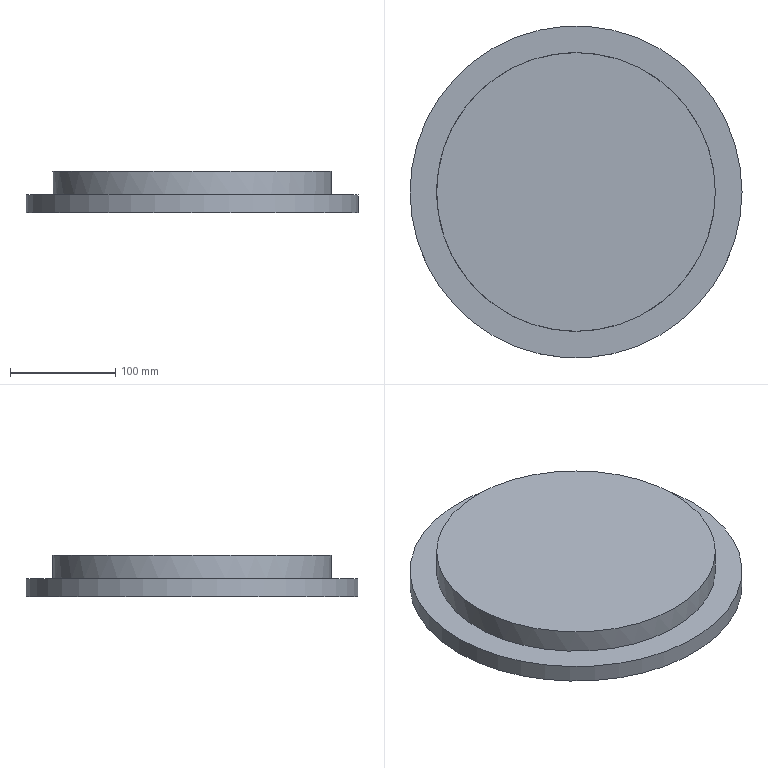Part | NX | features CYLINDER 3, DATUM_CSYS 1, Delete Body 1, LINKED_BODY 1, SCALE 1, UNITE 1 | 1 solid | 7 faces | box 315 x 315 x 39.375 mm | volume 2172802 mm3 | plane 4 | cylinder 3 | commonest cylinder face diameters 168.75 x1 264.375 x1 315 x1
STEP:
#1=CARTESIAN_POINT('',(-234.395,-2029.479,187.25));
#2=VERTEX_POINT('',#1);
#3=CARTESIAN_POINT('',(-366.582,-2029.479,187.25));
#4=DIRECTION('',(0.,0.,1.));
#5=DIRECTION('',(1.,0.,0.));
#6=AXIS2_PLACEMENT_3D('',#3,#4,#5);
#7=CIRCLE('',#6,132.188);
#8=EDGE_CURVE('',#2,#2,#7,.T.);
#9=ORIENTED_EDGE('',*,*,#8,.F.);
#10=EDGE_LOOP('',(#9));
#11=FACE_BOUND('',#10,.T.);
#12=CARTESIAN_POINT('',(-524.082,-2029.479,187.25));
#13=VERTEX_POINT('',#12);
#14=CARTESIAN_POINT('',(-366.582,-2029.479,187.25));
#15=DIRECTION('',(0.,0.,-1.));
#16=DIRECTION('',(-1.,0.,0.));
#17=AXIS2_PLACEMENT_3D('',#14,#15,#16);
#18=CIRCLE('',#17,157.5);
#19=EDGE_CURVE('',#13,#13,#18,.T.);
#20=ORIENTED_EDGE('',*,*,#19,.F.);
#21=EDGE_LOOP('',(#20));
#22=FACE_BOUND('',#21,.T.);
#23=CARTESIAN_POINT('',(-366.582,-2029.479,187.25));
#24=DIRECTION('',(0.,0.,1.));
#25=DIRECTION('',(1.,0.,0.));
#26=AXIS2_PLACEMENT_3D('',#23,#24,#25);
#27=PLANE('',#26);
#28=ADVANCED_FACE('',(#11,#22),#27,.T.);
#29=CARTESIAN_POINT('',(-282.207,-2029.479,170.375));
#30=VERTEX_POINT('',#29);
#31=CARTESIAN_POINT('',(-366.582,-2029.479,170.375));
#32=DIRECTION('',(0.,0.,1.));
#33=DIRECTION('',(1.,0.,0.));
#34=AXIS2_PLACEMENT_3D('',#31,#32,#33);
#35=CIRCLE('',#34,84.375);
#36=EDGE_CURVE('',#30,#30,#35,.T.);
#37=ORIENTED_EDGE('',*,*,#36,.T.);
#38=EDGE_LOOP('',(#37));
#39=FACE_BOUND('',#38,.T.);
#40=CARTESIAN_POINT('',(-209.082,-2029.479,170.375));
#41=VERTEX_POINT('',#40);
#42=CARTESIAN_POINT('',(-366.582,-2029.479,170.375));
#43=DIRECTION('',(0.,0.,1.));
#44=DIRECTION('',(1.,0.,0.));
#45=AXIS2_PLACEMENT_3D('',#42,#43,#44);
#46=CIRCLE('',#45,157.5);
#47=EDGE_CURVE('',#41,#41,#46,.T.);
#48=ORIENTED_EDGE('',*,*,#47,.F.);
#49=EDGE_LOOP('',(#48));
#50=FACE_BOUND('',#49,.T.);
#51=CARTESIAN_POINT('',(-366.582,-2029.479,170.375));
#52=DIRECTION('',(0.,0.,-1.));
#53=DIRECTION('',(-1.,0.,0.));
#54=AXIS2_PLACEMENT_3D('',#51,#52,#53);
#55=PLANE('',#54);
#56=ADVANCED_FACE('',(#39,#50),#55,.T.);
#57=ORIENTED_EDGE('',*,*,#19,.T.);
#58=EDGE_LOOP('',(#57));
#59=FACE_BOUND('',#58,.T.);
#60=ORIENTED_EDGE('',*,*,#47,.T.);
#61=EDGE_LOOP('',(#60));
#62=FACE_BOUND('',#61,.T.);
#63=CARTESIAN_POINT('',(-366.582,-2029.479,170.375));
#64=DIRECTION('',(0.,0.,1.));
#65=DIRECTION('',(1.,0.,0.));
#66=AXIS2_PLACEMENT_3D('',#63,#64,#65);
#67=CYLINDRICAL_SURFACE('',#66,157.5);
#68=ADVANCED_FACE('',(#59,#62),#67,.T.);
#69=CARTESIAN_POINT('',(-498.77,-2029.479,209.75));
#70=VERTEX_POINT('',#69);
#71=CARTESIAN_POINT('',(-366.582,-2029.479,209.75));
#72=DIRECTION('',(0.,0.,-1.));
#73=DIRECTION('',(-1.,0.,0.));
#74=AXIS2_PLACEMENT_3D('',#71,#72,#73);
#75=CIRCLE('',#74,132.188);
#76=EDGE_CURVE('',#70,#70,#75,.T.);
#77=ORIENTED_EDGE('',*,*,#76,.F.);
#78=EDGE_LOOP('',(#77));
#79=FACE_BOUND('',#78,.T.);
#80=CARTESIAN_POINT('',(-366.582,-2029.479,209.75));
#81=DIRECTION('',(0.,0.,1.));
#82=DIRECTION('',(1.,0.,0.));
#83=AXIS2_PLACEMENT_3D('',#80,#81,#82);
#84=PLANE('',#83);
#85=ADVANCED_FACE('',(#79),#84,.T.);
#86=ORIENTED_EDGE('',*,*,#8,.T.);
#87=EDGE_LOOP('',(#86));
#88=FACE_BOUND('',#87,.T.);
#89=ORIENTED_EDGE('',*,*,#76,.T.);
#90=EDGE_LOOP('',(#89));
#91=FACE_BOUND('',#90,.T.);
#92=CARTESIAN_POINT('',(-366.582,-2029.479,170.375));
#93=DIRECTION('',(0.,0.,1.));
#94=DIRECTION('',(1.,0.,0.));
#95=AXIS2_PLACEMENT_3D('',#92,#93,#94);
#96=CYLINDRICAL_SURFACE('',#95,132.188);
#97=ADVANCED_FACE('',(#88,#91),#96,.T.);
#98=CARTESIAN_POINT('',(-450.957,-2029.479,187.25));
#99=VERTEX_POINT('',#98);
#100=CARTESIAN_POINT('',(-366.582,-2029.479,187.25));
#101=DIRECTION('',(0.,0.,-1.));
#102=DIRECTION('',(-1.,0.,0.));
#103=AXIS2_PLACEMENT_3D('',#100,#101,#102);
#104=CIRCLE('',#103,84.375);
#105=EDGE_CURVE('',#99,#99,#104,.F.);
#106=ORIENTED_EDGE('',*,*,#105,.F.);
#107=EDGE_LOOP('',(#106));
#108=FACE_BOUND('',#107,.T.);
#109=CARTESIAN_POINT('',(-366.582,-2029.479,187.25));
#110=DIRECTION('',(0.,0.,1.));
#111=DIRECTION('',(1.,0.,0.));
#112=AXIS2_PLACEMENT_3D('',#109,#110,#111);
#113=PLANE('',#112);
#114=ADVANCED_FACE('',(#108),#113,.F.);
#115=ORIENTED_EDGE('',*,*,#105,.T.);
#116=EDGE_LOOP('',(#115));
#117=FACE_BOUND('',#116,.T.);
#118=ORIENTED_EDGE('',*,*,#36,.F.);
#119=EDGE_LOOP('',(#118));
#120=FACE_BOUND('',#119,.T.);
#121=CARTESIAN_POINT('',(-366.582,-2029.479,170.375));
#122=DIRECTION('',(0.,0.,1.));
#123=DIRECTION('',(1.,0.,0.));
#124=AXIS2_PLACEMENT_3D('',#121,#122,#123);
#125=CYLINDRICAL_SURFACE('',#124,84.375);
#126=ADVANCED_FACE('',(#117,#120),#125,.F.);
#127=CLOSED_SHELL('',(#28,#56,#68,#85,#97,#114,#126));
#128=MANIFOLD_SOLID_BREP('',#127);
#129=(LENGTH_UNIT()NAMED_UNIT(*)SI_UNIT(.MILLI.,.METRE.));
#130=UNCERTAINTY_MEASURE_WITH_UNIT(LENGTH_MEASURE(0.00001),#129,'','');
#131=(NAMED_UNIT(*)PLANE_ANGLE_UNIT()SI_UNIT($,.RADIAN.));
#132=(NAMED_UNIT(*)SI_UNIT($,.STERADIAN.)SOLID_ANGLE_UNIT());
#133=(GEOMETRIC_REPRESENTATION_CONTEXT(3)GLOBAL_UNCERTAINTY_ASSIGNED_CONTEXT((#130))GLOBAL_UNIT_ASSIGNED_CONTEXT((#129,#131,#132))REPRESENTATION_CONTEXT('',''));
#134=ADVANCED_BREP_SHAPE_REPRESENTATION('',(#128),#133);